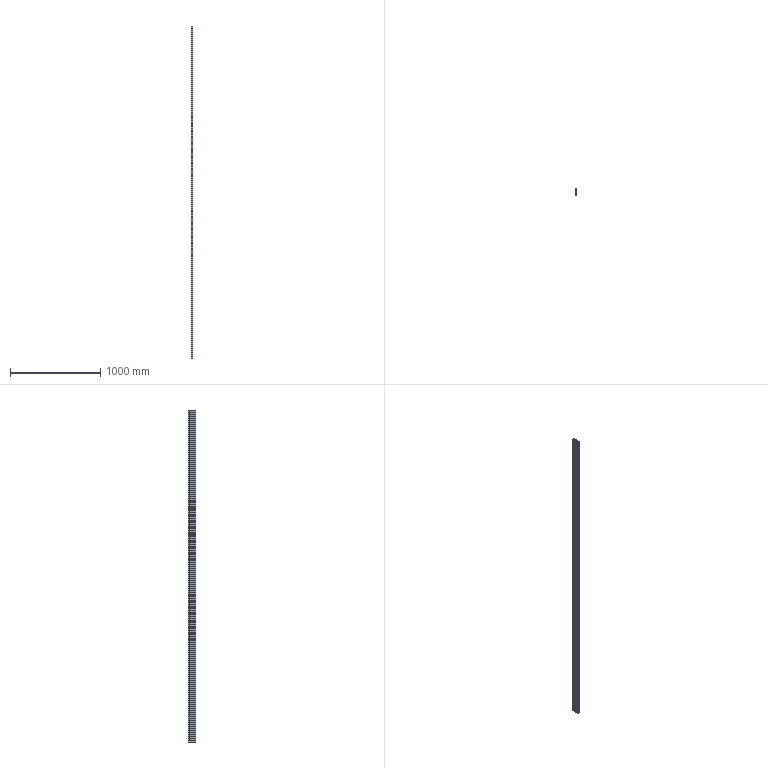Part | STEP file | New 20APBM1303-03_HFS5-2080-1380 | 1 solid | 356 faces | box 20 x 80 x 3680 mm | volume 2231978 mm3 | plane 244 | cylinder 112 | commonest cylinder face diameters 0.6 x36 10 x32 4.2 x24 5.5 x16 2 x4